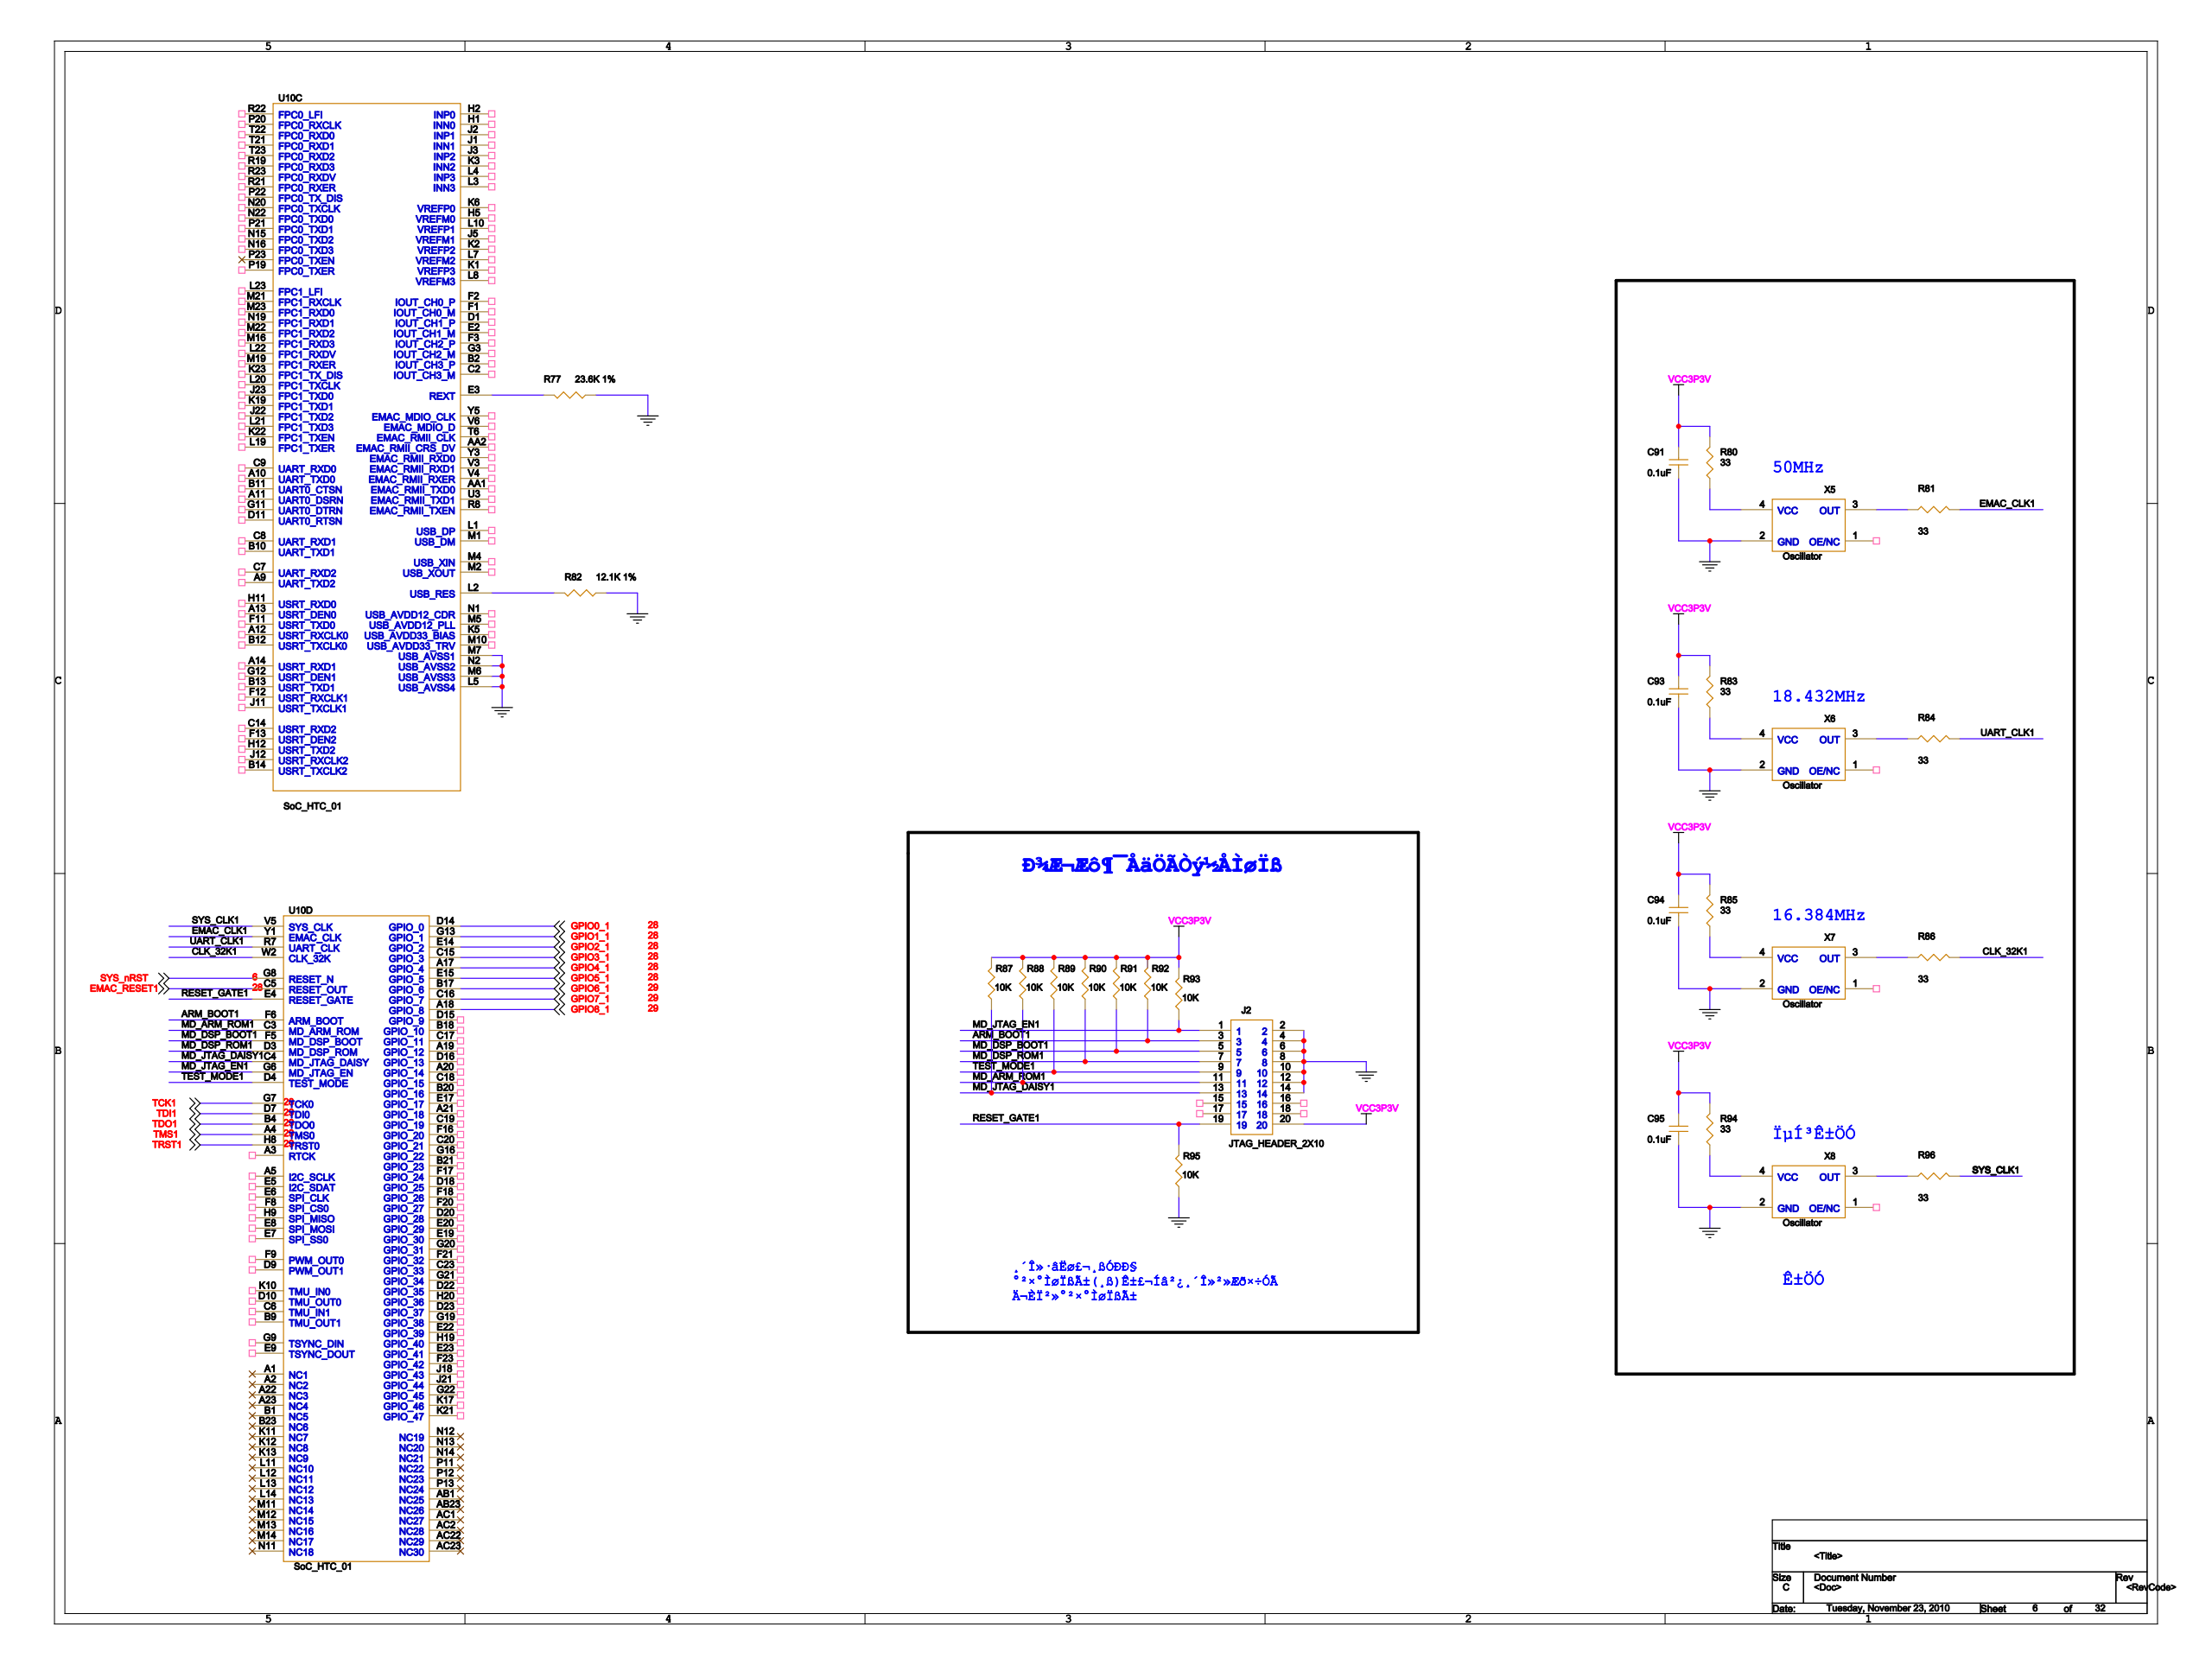Circuit board | Cadence Allegro | 1001 parts | 1318 nets | one sheet of the schematic
Parts on this sheet (reference | value | footprint):
C91 | 0.1uF | 0603
C93 | 0.1uF | 0603
C94 | 0.1uF | 0603
C95 | 0.1uF | 0603
J2 | JTAG_HEADER_2X10 | JTAG_HEADER_2X10
R77 | 23.6K 1% | 0603
R80 | 33 | 0603
R81 | 33 | 0603
R82 | 12.1K 1% | 0603
R83 | 33 | 0603
R84 | 33 | 0603
R85 | 33 | 0603
R86 | 33 | 0603
R87 | 10K | 0603
R88 | 10K | 0603
R89 | 10K | 0603
R90 | 10K | 0603
R91 | 10K | 0603
R92 | 10K | 0603
R93 | 10K | 0603
R94 | 33 | 0603
R95 | 10K | 0603
R96 | 33 | 0603
U10 | SoC_HTC_01 | L529_XIN
X5 | Oscillator | OSC_5_7
X6 | Oscillator | OSC_5_7
X7 | Oscillator | OSC_5_7
X8 | Oscillator | OSC_5_7
Nets of these parts (net: part-pin ...):
GPIO6_1: U10-B17
GPIO8_1: U10-A18
GPIO4_1: U10-A17
GPIO7_1: U10-C16
EMAC_RESET1: U10-C5
TMS1: U10-A4
GPIO2_1: U10-E14
GPIO0_1: U10-D14
TDO1: U10-B4
GPIO1_1: U10-G13
GPIO3_1: U10-C15
GPIO5_1: U10-E15
TRST1: U10-H8
TDI1: U10-D7
TCK1: U10-G7
GND: C91-2 C93-2 C94-2 C95-2 J2-2 J2-4 J2-6 J2-8 J2-10 J2-12 J2-14 R77-1 R82-1 R95-1 X5-2 X6-2 X7-2 X8-2 U10-L5 U10-M6 U10-M7 U10-N2
VCC3P3V: C91-1 C93-1 C94-1 C95-1 J2-20 R80-2 R83-2 R85-2 R87-2 R88-2 R89-2 R90-2 R91-2 R92-2 R93-2 R94-2
N16699736: R77-2 U10-E3
N16700218: R82-2 U10-L2
ARM_BOOT1: J2-3 R92-1 U10-F6
CLK_32K1: R86-2 U10-W2
EMAC_CLK1: R81-2 U10-Y1
MD_ARM_ROM1: J2-11 R88-1 U10-C3
MD_DSP_BOOT1: J2-5 R91-1 U10-F5
MD_DSP_ROM1: J2-7 R90-1 U10-D3
MD_JTAG_DAISY1: J2-13 R87-1 U10-C4
MD_JTAG_EN1: J2-1 R93-1 U10-G6
RESET_GATE1: J2-19 R95-2 U10-E4
SYS_CLK_16699576: R96-2 U10-V5
TEST_MODE1: J2-9 R89-1 U10-D4
UART_CLK1: R84-2 U10-R7
N16702042: R80-1 X5-4
N16702086: R81-1 X5-3
N16702128: R83-1 X6-4
N16702152: R84-1 X6-3
N16702440: R85-1 X7-4
N16702486: R86-1 X7-3
N16702528: R94-1 X8-4
N16702566: R96-1 X8-3